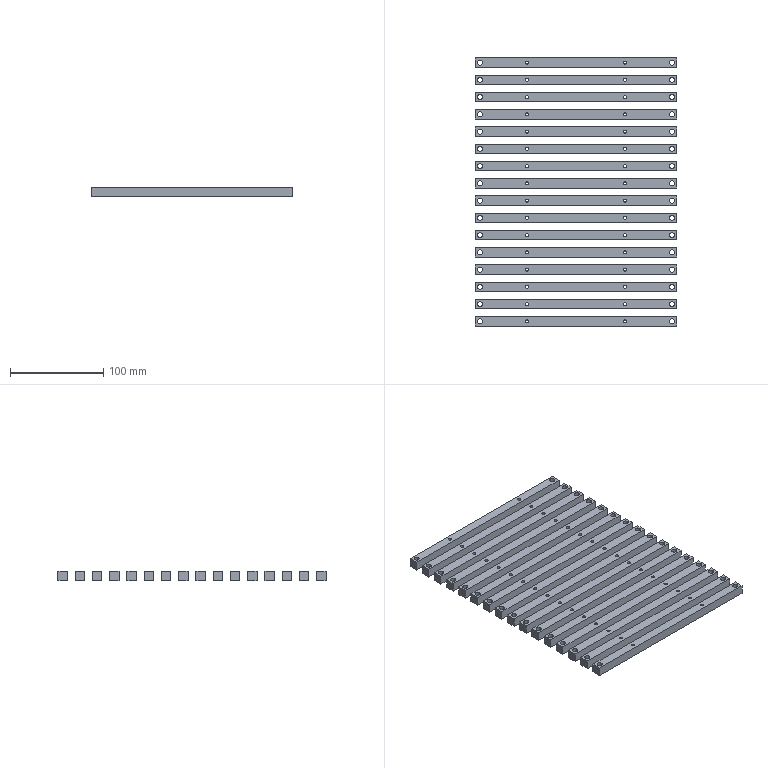Part | 16 solids | 224 faces | box 216 x 287.5 x 10 mm | volume 335260 mm3 | cylinder 128 | plane 96 | commonest cylinder face diameters 3.3 x64 5.5 x64